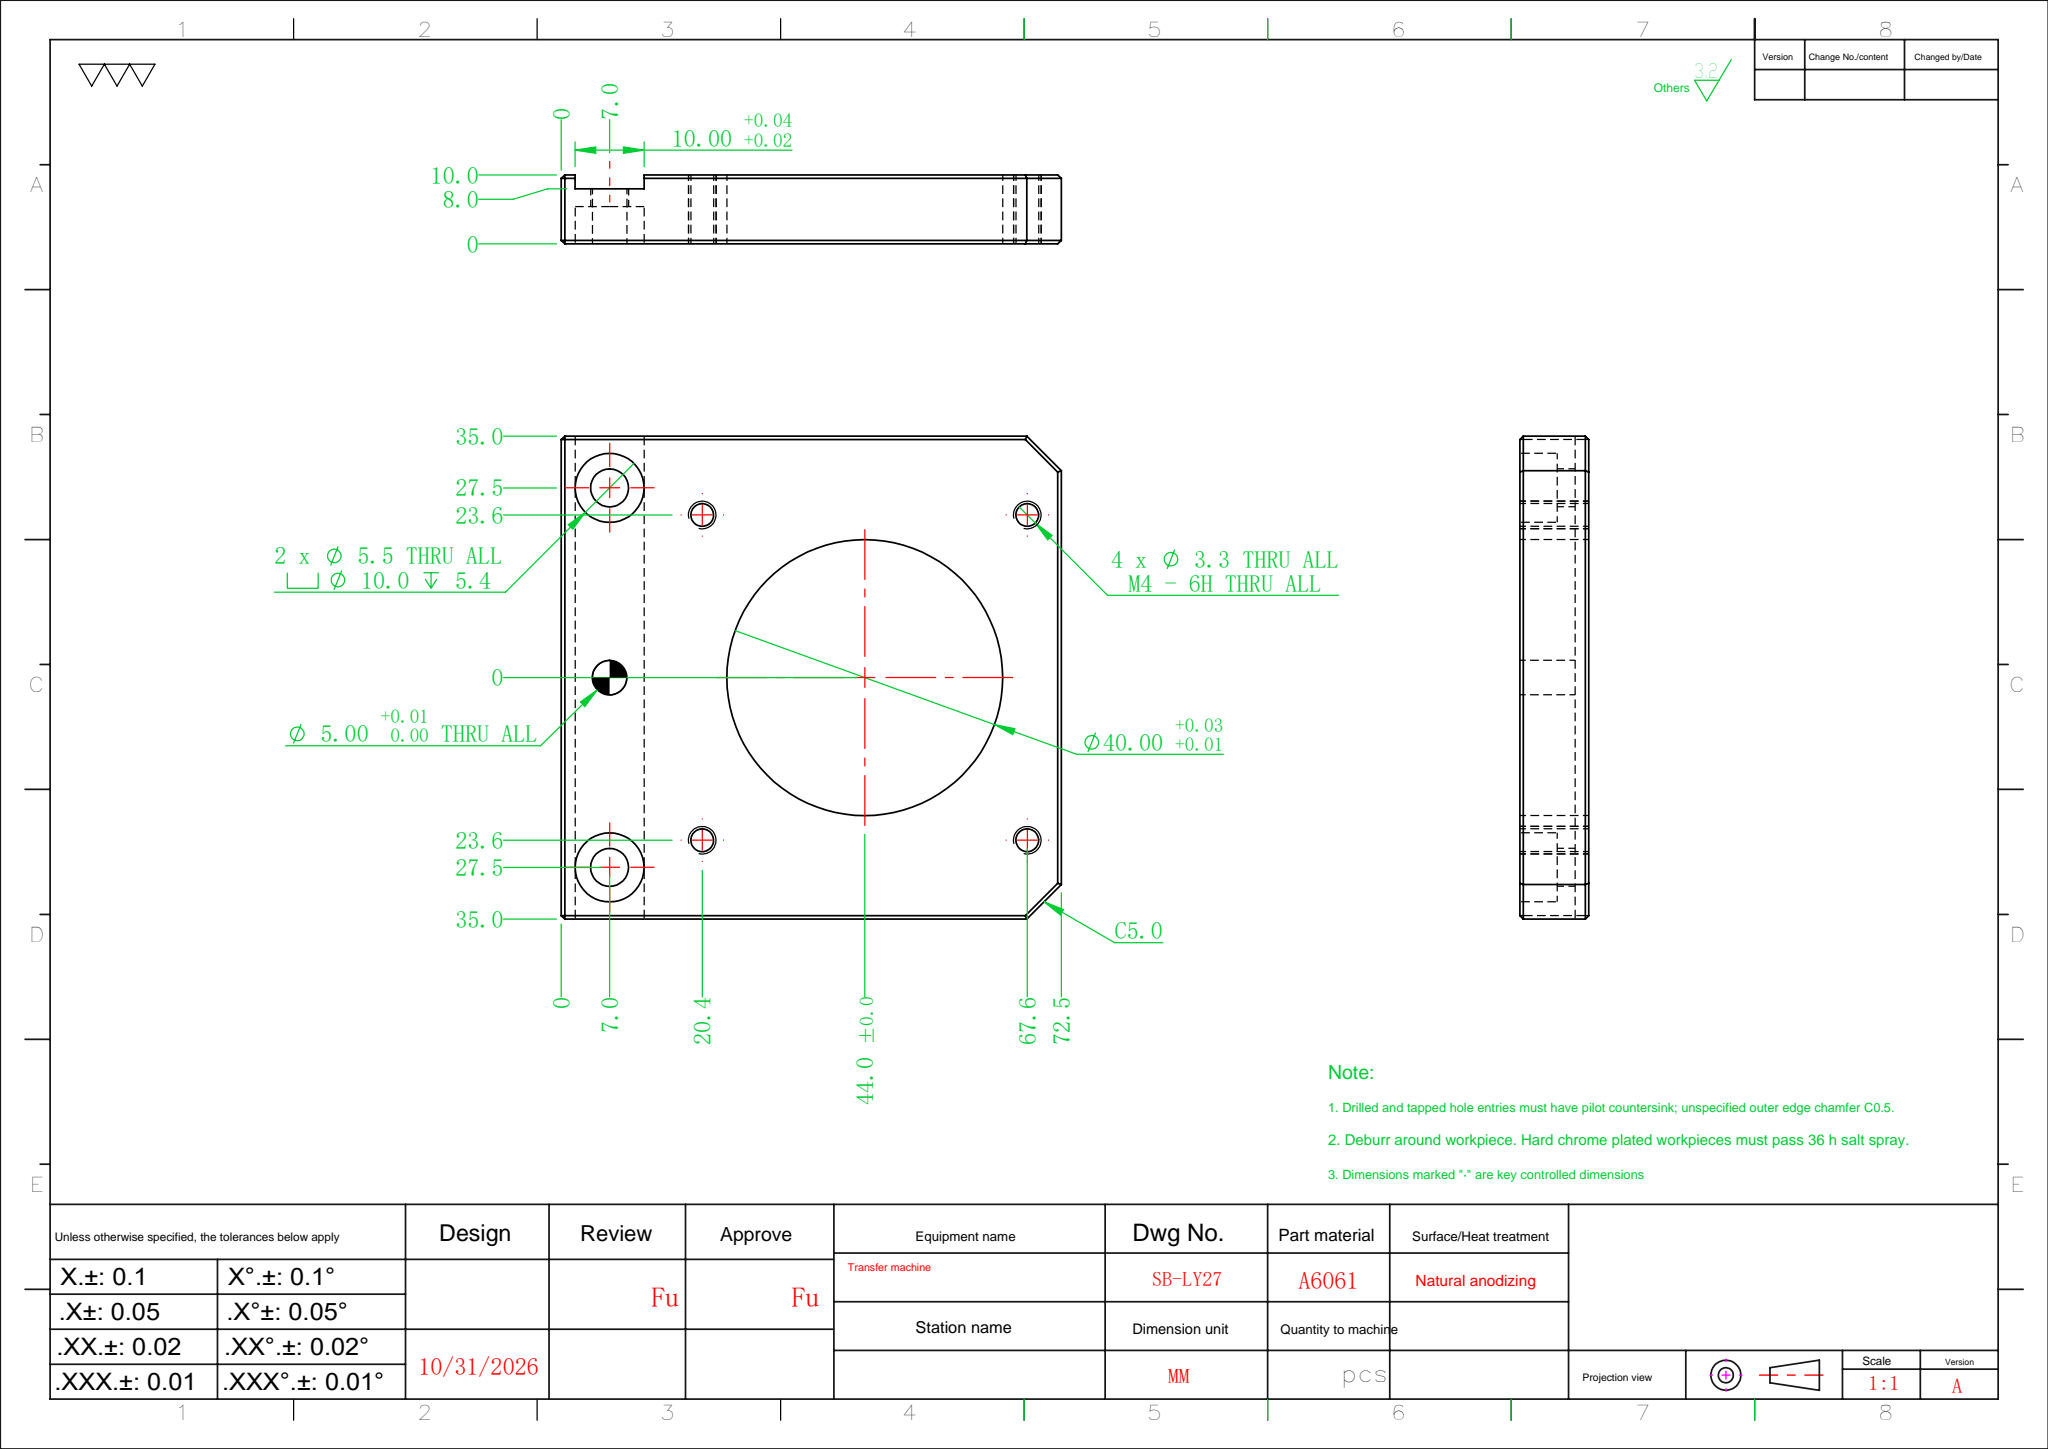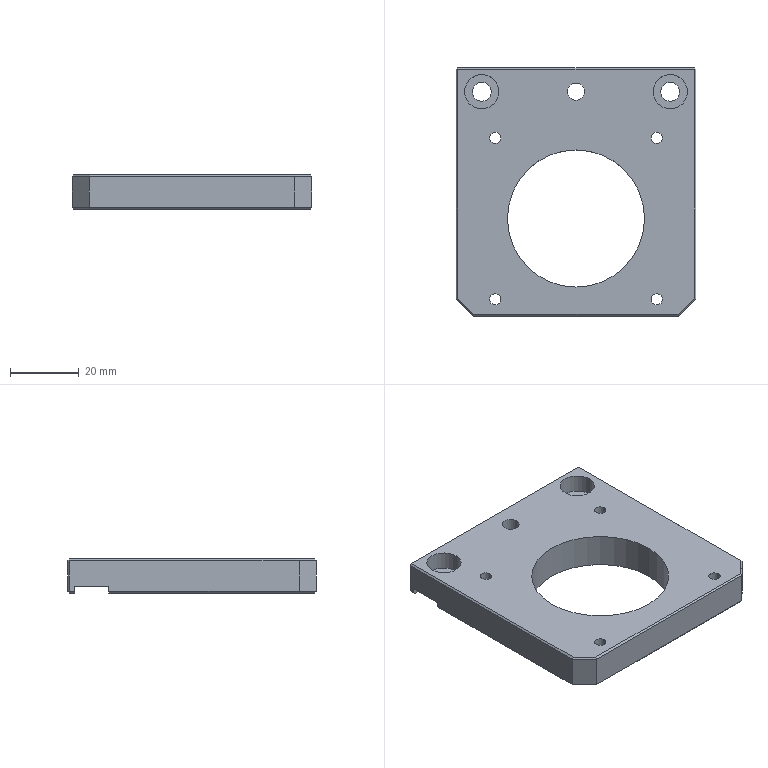Part | SolidWorks | features HoleWzd 3, Chamfer 2, Cut 2, Extrusion 1 | 1 solid | 54 faces | box 70 x 72.5 x 10 mm | volume 34993 mm3 | plane 34 | cylinder 20 | commonest cylinder face diameters 3.3 x8 5.5 x4 10 x4 5 x2 40 x2